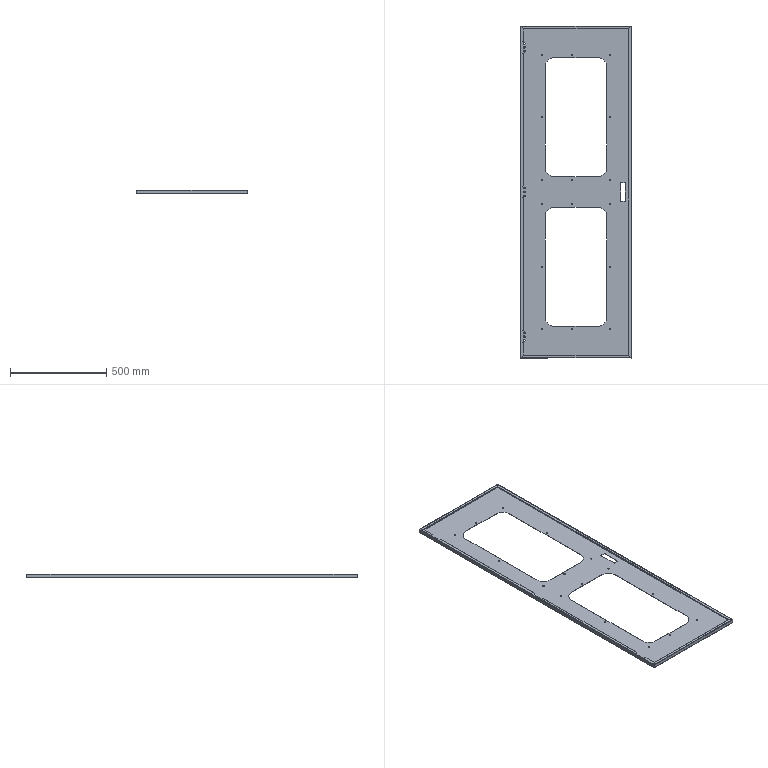Part | STEP file | Hinged door 1-right | 1 solid | 174 faces | box 574 x 1721 x 20 mm | volume 1096679 mm3 | cylinder 86 | plane 76 | spline 12 | commonest cylinder face diameters 7.5 x32 8.7 x18 0.4 x11 3.4 x11 100 x8 10 x6